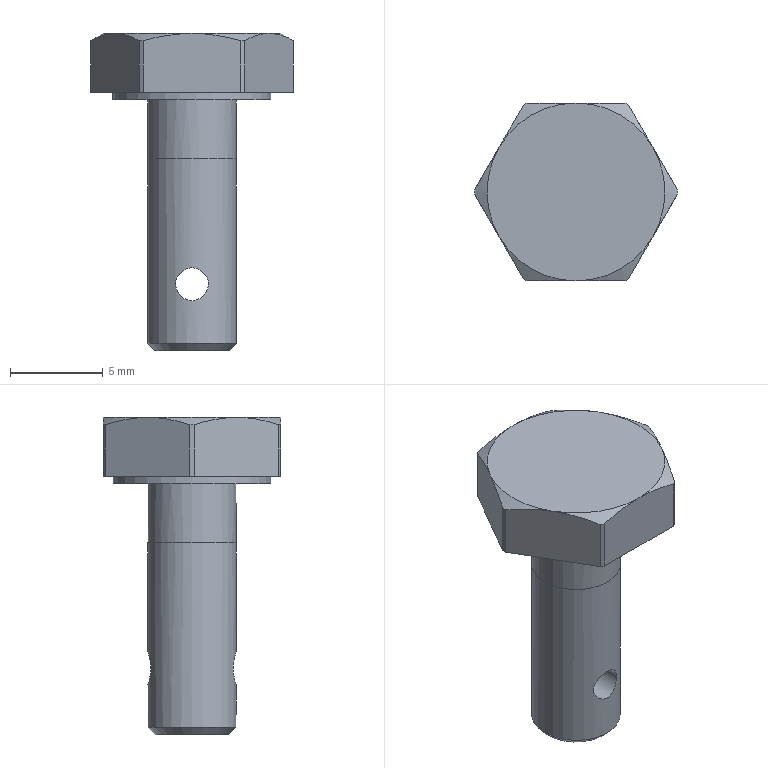Part | NX | features solid 2 | 1 solid | 27 faces | box 10.922 x 9.576 x 17.075 mm | volume 501.991 mm3 | cylinder 10 | plane 10 | cone 7 | commonest cylinder face diameters 10.922 x6 4.763 x2 1.778 x1 8.509 x1
STEP:
#1=CARTESIAN_POINT('',(0.,-2.381,-14.392));
#2=VERTEX_POINT('',#1);
#3=CARTESIAN_POINT('',(1.334,-2.037,-13.504));
#4=CARTESIAN_POINT('',(-0.00007358,-2.553,-14.836));
#5=CARTESIAN_POINT('',(-1.333,-2.037,-13.504));
#6=CARTESIAN_POINT('',(-0.0005145,-2.553,-12.169));
#7=CARTESIAN_POINT('',(1.334,-2.037,-13.504));
#8=CARTESIAN_POINT('',(-0.00007358,-2.553,-14.836));
#9=CARTESIAN_POINT('',(-1.333,-2.037,-13.504));
#10=B_SPLINE_CURVE_WITH_KNOTS('',3,(#3,#4,#5,#6,#7,#8,#9),.UNSPECIFIED.,.T.,.F.,(1,1,1,1,1,1,1,1,1,1,1),(-0.004207,-0.002805,-0.001402,0.,0.001402,0.002805,0.004207,0.00561,0.007012,0.008414,0.009817),.UNSPECIFIED.);
#11=EDGE_CURVE('',#2,#2,#10,.T.);
#12=ORIENTED_EDGE('',*,*,#11,.T.);
#13=EDGE_LOOP('',(#12));
#14=FACE_BOUND('',#13,.T.);
#15=CARTESIAN_POINT('',(-2.381,0.,-6.756));
#16=VERTEX_POINT('',#15);
#17=CARTESIAN_POINT('',(-1.866,1.866,-6.756));
#18=CARTESIAN_POINT('',(-2.639,0.,-6.756));
#19=CARTESIAN_POINT('',(-1.866,-1.866,-6.756));
#20=CARTESIAN_POINT('',(0.,-2.639,-6.756));
#21=CARTESIAN_POINT('',(1.866,-1.866,-6.756));
#22=CARTESIAN_POINT('',(2.639,0.,-6.756));
#23=CARTESIAN_POINT('',(1.866,1.866,-6.756));
#24=CARTESIAN_POINT('',(0.,2.639,-6.756));
#25=CARTESIAN_POINT('',(-1.866,1.866,-6.756));
#26=CARTESIAN_POINT('',(-2.639,0.,-6.756));
#27=CARTESIAN_POINT('',(-1.866,-1.866,-6.756));
#28=B_SPLINE_CURVE_WITH_KNOTS('',3,(#17,#18,#19,#20,#21,#22,#23,#24,#25,#26,#27),.UNSPECIFIED.,.T.,.F.,(1,1,1,1,1,1,1,1,1,1,1,1,1,1,1),(-0.375,-0.25,-0.125,0.,0.125,0.25,0.375,0.5,0.625,0.75,0.875,1.,1.125,1.25,1.375),.UNSPECIFIED.);
#29=EDGE_CURVE('',#16,#16,#28,.T.);
#30=ORIENTED_EDGE('',*,*,#29,.F.);
#31=EDGE_LOOP('',(#30));
#32=FACE_BOUND('',#31,.T.);
#33=CARTESIAN_POINT('',(-2.381,0.,-16.694));
#34=VERTEX_POINT('',#33);
#35=CARTESIAN_POINT('',(0.,0.,-16.694));
#36=DIRECTION('',(0.,0.,-1.));
#37=DIRECTION('',(-1.,0.,0.));
#38=AXIS2_PLACEMENT_3D('',#35,#36,#37);
#39=CIRCLE('',#38,2.381);
#40=EDGE_CURVE('',#34,#34,#39,.T.);
#41=ORIENTED_EDGE('',*,*,#40,.F.);
#42=EDGE_LOOP('',(#41));
#43=FACE_BOUND('',#42,.T.);
#44=CARTESIAN_POINT('',(0.,2.381,-14.392));
#45=VERTEX_POINT('',#44);
#46=CARTESIAN_POINT('',(-1.334,2.037,-13.504));
#47=CARTESIAN_POINT('',(0.00007358,2.553,-14.836));
#48=CARTESIAN_POINT('',(1.333,2.037,-13.504));
#49=CARTESIAN_POINT('',(0.0005145,2.553,-12.169));
#50=CARTESIAN_POINT('',(-1.334,2.037,-13.504));
#51=CARTESIAN_POINT('',(0.00007358,2.553,-14.836));
#52=CARTESIAN_POINT('',(1.333,2.037,-13.504));
#53=B_SPLINE_CURVE_WITH_KNOTS('',3,(#46,#47,#48,#49,#50,#51,#52),.UNSPECIFIED.,.T.,.F.,(1,1,1,1,1,1,1,1,1,1,1),(-0.004207,-0.002805,-0.001402,0.,0.001402,0.002805,0.004207,0.00561,0.007012,0.008414,0.009817),.UNSPECIFIED.);
#54=EDGE_CURVE('',#45,#45,#53,.T.);
#55=ORIENTED_EDGE('',*,*,#54,.T.);
#56=EDGE_LOOP('',(#55));
#57=FACE_BOUND('',#56,.T.);
#58=CARTESIAN_POINT('',(0.,0.,0.));
#59=DIRECTION('',(0.,0.,-1.));
#60=DIRECTION('',(-1.,0.,0.));
#61=AXIS2_PLACEMENT_3D('',#58,#59,#60);
#62=CYLINDRICAL_SURFACE('',#61,2.381);
#63=ADVANCED_FACE('',(#14,#32,#43,#57),#62,.T.);
#64=CARTESIAN_POINT('',(-2.381,0.,-3.581));
#65=VERTEX_POINT('',#64);
#66=CARTESIAN_POINT('',(0.,0.,-3.581));
#67=DIRECTION('',(0.,0.,-1.));
#68=DIRECTION('',(-1.,0.,0.));
#69=AXIS2_PLACEMENT_3D('',#66,#67,#68);
#70=CIRCLE('',#69,2.381);
#71=EDGE_CURVE('',#65,#65,#70,.T.);
#72=ORIENTED_EDGE('',*,*,#71,.T.);
#73=EDGE_LOOP('',(#72));
#74=FACE_BOUND('',#73,.T.);
#75=ORIENTED_EDGE('',*,*,#29,.T.);
#76=EDGE_LOOP('',(#75));
#77=FACE_BOUND('',#76,.T.);
#78=CARTESIAN_POINT('',(0.,0.,0.));
#79=DIRECTION('',(0.,0.,-1.));
#80=DIRECTION('',(-1.,0.,0.));
#81=AXIS2_PLACEMENT_3D('',#78,#79,#80);
#82=CYLINDRICAL_SURFACE('',#81,2.381);
#83=ADVANCED_FACE('',(#74,#77),#82,.T.);
#84=CARTESIAN_POINT('',(2.627,4.788,-3.175));
#85=VERTEX_POINT('',#84);
#86=CARTESIAN_POINT('',(2.833,4.669,-3.175));
#87=VERTEX_POINT('',#86);
#88=CARTESIAN_POINT('',(0.,0.,-3.175));
#89=DIRECTION('',(0.,0.,-1.));
#90=DIRECTION('',(-1.,0.,0.));
#91=AXIS2_PLACEMENT_3D('',#88,#89,#90);
#92=CIRCLE('',#91,5.461);
#93=EDGE_CURVE('',#85,#87,#92,.T.);
#94=ORIENTED_EDGE('',*,*,#93,.F.);
#95=CARTESIAN_POINT('',(2.627,4.788,-0.3886));
#96=VERTEX_POINT('',#95);
#97=CARTESIAN_POINT('',(2.627,4.788,0.));
#98=DIRECTION('',(0.,0.,-1.));
#99=VECTOR('',#98,1000.);
#100=LINE('',#97,#99);
#101=EDGE_CURVE('',#85,#96,#100,.F.);
#102=ORIENTED_EDGE('',*,*,#101,.T.);
#103=CARTESIAN_POINT('',(2.833,4.669,-0.3886));
#104=VERTEX_POINT('',#103);
#105=CARTESIAN_POINT('',(0.,0.,-0.3886));
#106=DIRECTION('',(0.,0.,-1.));
#107=DIRECTION('',(-1.,0.,0.));
#108=AXIS2_PLACEMENT_3D('',#105,#106,#107);
#109=CIRCLE('',#108,5.461);
#110=EDGE_CURVE('',#96,#104,#109,.T.);
#111=ORIENTED_EDGE('',*,*,#110,.T.);
#112=CARTESIAN_POINT('',(2.833,4.669,0.));
#113=DIRECTION('',(0.,0.,-1.));
#114=VECTOR('',#113,1000.);
#115=LINE('',#112,#114);
#116=EDGE_CURVE('',#104,#87,#115,.T.);
#117=ORIENTED_EDGE('',*,*,#116,.T.);
#118=EDGE_LOOP('',(#94,#102,#111,#117));
#119=FACE_BOUND('',#118,.T.);
#120=CARTESIAN_POINT('',(0.,0.,0.));
#121=DIRECTION('',(0.,0.,-1.));
#122=DIRECTION('',(-1.,0.,0.));
#123=AXIS2_PLACEMENT_3D('',#120,#121,#122);
#124=CYLINDRICAL_SURFACE('',#123,5.461);
#125=ADVANCED_FACE('',(#119),#124,.T.);
#126=CARTESIAN_POINT('',(-2.833,4.669,-0.3886));
#127=VERTEX_POINT('',#126);
#128=CARTESIAN_POINT('',(-2.627,4.788,-0.3886));
#129=VERTEX_POINT('',#128);
#130=CARTESIAN_POINT('',(0.,0.,-0.3886));
#131=DIRECTION('',(0.,0.,-1.));
#132=DIRECTION('',(-1.,0.,0.));
#133=AXIS2_PLACEMENT_3D('',#130,#131,#132);
#134=CIRCLE('',#133,5.461);
#135=EDGE_CURVE('',#127,#129,#134,.T.);
#136=ORIENTED_EDGE('',*,*,#135,.T.);
#137=CARTESIAN_POINT('',(-2.627,4.788,-3.175));
#138=VERTEX_POINT('',#137);
#139=CARTESIAN_POINT('',(-2.627,4.788,0.));
#140=DIRECTION('',(0.,0.,-1.));
#141=VECTOR('',#140,1000.);
#142=LINE('',#139,#141);
#143=EDGE_CURVE('',#129,#138,#142,.T.);
#144=ORIENTED_EDGE('',*,*,#143,.T.);
#145=CARTESIAN_POINT('',(-2.833,4.669,-3.175));
#146=VERTEX_POINT('',#145);
#147=CARTESIAN_POINT('',(0.,0.,-3.175));
#148=DIRECTION('',(0.,0.,-1.));
#149=DIRECTION('',(-1.,0.,0.));
#150=AXIS2_PLACEMENT_3D('',#147,#148,#149);
#151=CIRCLE('',#150,5.461);
#152=EDGE_CURVE('',#146,#138,#151,.T.);
#153=ORIENTED_EDGE('',*,*,#152,.F.);
#154=CARTESIAN_POINT('',(-2.833,4.669,0.));
#155=DIRECTION('',(0.,0.,-1.));
#156=VECTOR('',#155,1000.);
#157=LINE('',#154,#156);
#158=EDGE_CURVE('',#146,#127,#157,.F.);
#159=ORIENTED_EDGE('',*,*,#158,.T.);
#160=EDGE_LOOP('',(#136,#144,#153,#159));
#161=FACE_BOUND('',#160,.T.);
#162=CARTESIAN_POINT('',(0.,0.,0.));
#163=DIRECTION('',(0.,0.,-1.));
#164=DIRECTION('',(-1.,0.,0.));
#165=AXIS2_PLACEMENT_3D('',#162,#163,#164);
#166=CYLINDRICAL_SURFACE('',#165,5.461);
#167=ADVANCED_FACE('',(#161),#166,.T.);
#168=CARTESIAN_POINT('',(-5.46,-0.1193,-0.3886));
#169=VERTEX_POINT('',#168);
#170=CARTESIAN_POINT('',(-5.46,0.1193,-0.3886));
#171=VERTEX_POINT('',#170);
#172=CARTESIAN_POINT('',(0.,0.,-0.3886));
#173=DIRECTION('',(0.,0.,-1.));
#174=DIRECTION('',(-1.,0.,0.));
#175=AXIS2_PLACEMENT_3D('',#172,#173,#174);
#176=CIRCLE('',#175,5.461);
#177=EDGE_CURVE('',#169,#171,#176,.T.);
#178=ORIENTED_EDGE('',*,*,#177,.T.);
#179=CARTESIAN_POINT('',(-5.46,0.1193,-3.175));
#180=VERTEX_POINT('',#179);
#181=CARTESIAN_POINT('',(-5.46,0.1193,0.));
#182=DIRECTION('',(0.,0.,-1.));
#183=VECTOR('',#182,1000.);
#184=LINE('',#181,#183);
#185=EDGE_CURVE('',#171,#180,#184,.T.);
#186=ORIENTED_EDGE('',*,*,#185,.T.);
#187=CARTESIAN_POINT('',(-5.46,-0.1193,-3.175));
#188=VERTEX_POINT('',#187);
#189=CARTESIAN_POINT('',(0.,0.,-3.175));
#190=DIRECTION('',(0.,0.,-1.));
#191=DIRECTION('',(-1.,0.,0.));
#192=AXIS2_PLACEMENT_3D('',#189,#190,#191);
#193=CIRCLE('',#192,5.461);
#194=EDGE_CURVE('',#188,#180,#193,.T.);
#195=ORIENTED_EDGE('',*,*,#194,.F.);
#196=CARTESIAN_POINT('',(-5.46,-0.1193,0.));
#197=DIRECTION('',(0.,0.,-1.));
#198=VECTOR('',#197,1000.);
#199=LINE('',#196,#198);
#200=EDGE_CURVE('',#188,#169,#199,.F.);
#201=ORIENTED_EDGE('',*,*,#200,.T.);
#202=EDGE_LOOP('',(#178,#186,#195,#201));
#203=FACE_BOUND('',#202,.T.);
#204=CARTESIAN_POINT('',(0.,0.,0.));
#205=DIRECTION('',(0.,0.,-1.));
#206=DIRECTION('',(-1.,0.,0.));
#207=AXIS2_PLACEMENT_3D('',#204,#205,#206);
#208=CYLINDRICAL_SURFACE('',#207,5.461);
#209=ADVANCED_FACE('',(#203),#208,.T.);
#210=CARTESIAN_POINT('',(-2.627,-4.788,-0.3886));
#211=VERTEX_POINT('',#210);
#212=CARTESIAN_POINT('',(-2.833,-4.669,-0.3886));
#213=VERTEX_POINT('',#212);
#214=CARTESIAN_POINT('',(0.,0.,-0.3886));
#215=DIRECTION('',(0.,0.,-1.));
#216=DIRECTION('',(-1.,0.,0.));
#217=AXIS2_PLACEMENT_3D('',#214,#215,#216);
#218=CIRCLE('',#217,5.461);
#219=EDGE_CURVE('',#211,#213,#218,.T.);
#220=ORIENTED_EDGE('',*,*,#219,.T.);
#221=CARTESIAN_POINT('',(-2.833,-4.669,-3.175));
#222=VERTEX_POINT('',#221);
#223=CARTESIAN_POINT('',(-2.833,-4.669,0.));
#224=DIRECTION('',(0.,0.,-1.));
#225=VECTOR('',#224,1000.);
#226=LINE('',#223,#225);
#227=EDGE_CURVE('',#213,#222,#226,.T.);
#228=ORIENTED_EDGE('',*,*,#227,.T.);
#229=CARTESIAN_POINT('',(-2.627,-4.788,-3.175));
#230=VERTEX_POINT('',#229);
#231=CARTESIAN_POINT('',(0.,0.,-3.175));
#232=DIRECTION('',(0.,0.,-1.));
#233=DIRECTION('',(-1.,0.,0.));
#234=AXIS2_PLACEMENT_3D('',#231,#232,#233);
#235=CIRCLE('',#234,5.461);
#236=EDGE_CURVE('',#230,#222,#235,.T.);
#237=ORIENTED_EDGE('',*,*,#236,.F.);
#238=CARTESIAN_POINT('',(-2.627,-4.788,0.));
#239=DIRECTION('',(0.,0.,-1.));
#240=VECTOR('',#239,1000.);
#241=LINE('',#238,#240);
#242=EDGE_CURVE('',#230,#211,#241,.F.);
#243=ORIENTED_EDGE('',*,*,#242,.T.);
#244=EDGE_LOOP('',(#220,#228,#237,#243));
#245=FACE_BOUND('',#244,.T.);
#246=CARTESIAN_POINT('',(0.,0.,0.));
#247=DIRECTION('',(0.,0.,-1.));
#248=DIRECTION('',(-1.,0.,0.));
#249=AXIS2_PLACEMENT_3D('',#246,#247,#248);
#250=CYLINDRICAL_SURFACE('',#249,5.461);
#251=ADVANCED_FACE('',(#245),#250,.T.);
#252=CARTESIAN_POINT('',(2.833,-4.669,-0.3886));
#253=VERTEX_POINT('',#252);
#254=CARTESIAN_POINT('',(2.627,-4.788,-0.3886));
#255=VERTEX_POINT('',#254);
#256=CARTESIAN_POINT('',(0.,0.,-0.3886));
#257=DIRECTION('',(0.,0.,-1.));
#258=DIRECTION('',(-1.,0.,0.));
#259=AXIS2_PLACEMENT_3D('',#256,#257,#258);
#260=CIRCLE('',#259,5.461);
#261=EDGE_CURVE('',#253,#255,#260,.T.);
#262=ORIENTED_EDGE('',*,*,#261,.T.);
#263=CARTESIAN_POINT('',(2.627,-4.788,-3.175));
#264=VERTEX_POINT('',#263);
#265=CARTESIAN_POINT('',(2.627,-4.788,0.));
#266=DIRECTION('',(0.,0.,-1.));
#267=VECTOR('',#266,1000.);
#268=LINE('',#265,#267);
#269=EDGE_CURVE('',#255,#264,#268,.T.);
#270=ORIENTED_EDGE('',*,*,#269,.T.);
#271=CARTESIAN_POINT('',(2.833,-4.669,-3.175));
#272=VERTEX_POINT('',#271);
#273=CARTESIAN_POINT('',(0.,0.,-3.175));
#274=DIRECTION('',(0.,0.,-1.));
#275=DIRECTION('',(-1.,0.,0.));
#276=AXIS2_PLACEMENT_3D('',#273,#274,#275);
#277=CIRCLE('',#276,5.461);
#278=EDGE_CURVE('',#272,#264,#277,.T.);
#279=ORIENTED_EDGE('',*,*,#278,.F.);
#280=CARTESIAN_POINT('',(2.833,-4.669,0.));
#281=DIRECTION('',(0.,0.,-1.));
#282=VECTOR('',#281,1000.);
#283=LINE('',#280,#282);
#284=EDGE_CURVE('',#272,#253,#283,.F.);
#285=ORIENTED_EDGE('',*,*,#284,.T.);
#286=EDGE_LOOP('',(#262,#270,#279,#285));
#287=FACE_BOUND('',#286,.T.);
#288=CARTESIAN_POINT('',(0.,0.,0.));
#289=DIRECTION('',(0.,0.,-1.));
#290=DIRECTION('',(-1.,0.,0.));
#291=AXIS2_PLACEMENT_3D('',#288,#289,#290);
#292=CYLINDRICAL_SURFACE('',#291,5.461);
#293=ADVANCED_FACE('',(#287),#292,.T.);
#294=ORIENTED_EDGE('',*,*,#110,.F.);
#295=CARTESIAN_POINT('',(0.,4.788,0.));
#296=VERTEX_POINT('',#295);
#297=CARTESIAN_POINT('',(0.,4.788,0.));
#298=CARTESIAN_POINT('',(0.8868,4.788,0.));
#299=CARTESIAN_POINT('',(1.776,4.788,-0.1525));
#300=CARTESIAN_POINT('',(2.627,4.788,-0.3886));
#301=B_SPLINE_CURVE_WITH_KNOTS('',3,(#297,#298,#299,#300),.UNSPECIFIED.,.F.,.F.,(4,4),(0.007722,0.01038),.UNSPECIFIED.);
#302=EDGE_CURVE('',#96,#296,#301,.F.);
#303=ORIENTED_EDGE('',*,*,#302,.T.);
#304=CARTESIAN_POINT('',(4.146,2.394,0.));
#305=VERTEX_POINT('',#304);
#306=CARTESIAN_POINT('',(0.,0.,0.));
#307=DIRECTION('',(0.,0.,-1.));
#308=DIRECTION('',(-1.,0.,0.));
#309=AXIS2_PLACEMENT_3D('',#306,#307,#308);
#310=CIRCLE('',#309,4.788);
#311=EDGE_CURVE('',#296,#305,#310,.T.);
#312=ORIENTED_EDGE('',*,*,#311,.T.);
#313=CARTESIAN_POINT('',(4.146,2.394,0.));
#314=CARTESIAN_POINT('',(3.703,3.163,0.));
#315=CARTESIAN_POINT('',(3.262,3.925,-0.1503));
#316=CARTESIAN_POINT('',(2.833,4.669,-0.3886));
#317=B_SPLINE_CURVE_WITH_KNOTS('',3,(#313,#314,#315,#316),.UNSPECIFIED.,.F.,.F.,(4,4),(0.002655,0.005296),.UNSPECIFIED.);
#318=EDGE_CURVE('',#305,#104,#317,.T.);
#319=ORIENTED_EDGE('',*,*,#318,.T.);
#320=EDGE_LOOP('',(#294,#303,#312,#319));
#321=FACE_BOUND('',#320,.T.);
#322=CARTESIAN_POINT('',(0.,0.,-0.3886));
#323=DIRECTION('',(0.,0.,-1.));
#324=DIRECTION('',(-1.,0.,0.));
#325=AXIS2_PLACEMENT_3D('',#322,#323,#324);
#326=CONICAL_SURFACE('',#325,5.461,1.047);
#327=ADVANCED_FACE('',(#321),#326,.T.);
#328=CARTESIAN_POINT('',(-4.146,2.394,0.));
#329=VERTEX_POINT('',#328);
#330=CARTESIAN_POINT('',(0.,0.,0.));
#331=DIRECTION('',(0.,0.,-1.));
#332=DIRECTION('',(-1.,0.,0.));
#333=AXIS2_PLACEMENT_3D('',#330,#331,#332);
#334=CIRCLE('',#333,4.788);
#335=EDGE_CURVE('',#329,#296,#334,.T.);
#336=ORIENTED_EDGE('',*,*,#335,.T.);
#337=CARTESIAN_POINT('',(-2.627,4.788,-0.3886));
#338=CARTESIAN_POINT('',(-1.77,4.788,-0.1508));
#339=CARTESIAN_POINT('',(-0.8866,4.788,0.));
#340=CARTESIAN_POINT('',(0.,4.788,0.));
#341=B_SPLINE_CURVE_WITH_KNOTS('',3,(#337,#338,#339,#340),.UNSPECIFIED.,.F.,.F.,(4,4),(0.005068,0.007722),.UNSPECIFIED.);
#342=EDGE_CURVE('',#296,#129,#341,.F.);
#343=ORIENTED_EDGE('',*,*,#342,.T.);
#344=ORIENTED_EDGE('',*,*,#135,.F.);
#345=CARTESIAN_POINT('',(-2.833,4.669,-0.3886));
#346=CARTESIAN_POINT('',(-3.264,3.923,-0.1495));
#347=CARTESIAN_POINT('',(-3.7,3.167,0.));
#348=CARTESIAN_POINT('',(-4.146,2.394,0.));
#349=B_SPLINE_CURVE_WITH_KNOTS('',3,(#345,#346,#347,#348),.UNSPECIFIED.,.F.,.F.,(4,4),(0.00000074,0.002655),.UNSPECIFIED.);
#350=EDGE_CURVE('',#127,#329,#349,.T.);
#351=ORIENTED_EDGE('',*,*,#350,.T.);
#352=EDGE_LOOP('',(#336,#343,#344,#351));
#353=FACE_BOUND('',#352,.T.);
#354=CARTESIAN_POINT('',(0.,0.,-0.3886));
#355=DIRECTION('',(0.,0.,-1.));
#356=DIRECTION('',(-1.,0.,0.));
#357=AXIS2_PLACEMENT_3D('',#354,#355,#356);
#358=CONICAL_SURFACE('',#357,5.461,1.047);
#359=ADVANCED_FACE('',(#353),#358,.T.);
#360=CARTESIAN_POINT('',(-4.146,-2.394,0.));
#361=VERTEX_POINT('',#360);
#362=CARTESIAN_POINT('',(0.,0.,0.));
#363=DIRECTION('',(0.,0.,-1.));
#364=DIRECTION('',(-1.,0.,0.));
#365=AXIS2_PLACEMENT_3D('',#362,#363,#364);
#366=CIRCLE('',#365,4.788);
#367=EDGE_CURVE('',#361,#329,#366,.T.);
#368=ORIENTED_EDGE('',*,*,#367,.T.);
#369=CARTESIAN_POINT('',(-4.146,2.394,0.));
#370=CARTESIAN_POINT('',(-4.59,1.625,0.));
#371=CARTESIAN_POINT('',(-5.031,0.8625,-0.1503));
#372=CARTESIAN_POINT('',(-5.46,0.1193,-0.3886));
#373=B_SPLINE_CURVE_WITH_KNOTS('',3,(#369,#370,#371,#372),.UNSPECIFIED.,.F.,.F.,(4,4),(0.002655,0.005296),.UNSPECIFIED.);
#374=EDGE_CURVE('',#329,#171,#373,.T.);
#375=ORIENTED_EDGE('',*,*,#374,.T.);
#376=ORIENTED_EDGE('',*,*,#177,.F.);
#377=CARTESIAN_POINT('',(-5.46,-0.1193,-0.3886));
#378=CARTESIAN_POINT('',(-5.029,-0.8651,-0.1495));
#379=CARTESIAN_POINT('',(-4.593,-1.621,0.));
#380=CARTESIAN_POINT('',(-4.146,-2.394,0.));
#381=B_SPLINE_CURVE_WITH_KNOTS('',3,(#377,#378,#379,#380),.UNSPECIFIED.,.F.,.F.,(4,4),(0.00000074,0.002655),.UNSPECIFIED.);
#382=EDGE_CURVE('',#169,#361,#381,.T.);
#383=ORIENTED_EDGE('',*,*,#382,.T.);
#384=EDGE_LOOP('',(#368,#375,#376,#383));
#385=FACE_BOUND('',#384,.T.);
#386=CARTESIAN_POINT('',(0.,0.,-0.3886));
#387=DIRECTION('',(0.,0.,-1.));
#388=DIRECTION('',(-1.,0.,0.));
#389=AXIS2_PLACEMENT_3D('',#386,#387,#388);
#390=CONICAL_SURFACE('',#389,5.461,1.047);
#391=ADVANCED_FACE('',(#385),#390,.T.);
#392=CARTESIAN_POINT('',(0.,-4.788,0.));
#393=VERTEX_POINT('',#392);
#394=CARTESIAN_POINT('',(0.,0.,0.));
#395=DIRECTION('',(0.,0.,-1.));
#396=DIRECTION('',(-1.,0.,0.));
#397=AXIS2_PLACEMENT_3D('',#394,#395,#396);
#398=CIRCLE('',#397,4.788);
#399=EDGE_CURVE('',#393,#361,#398,.T.);
#400=ORIENTED_EDGE('',*,*,#399,.T.);
#401=CARTESIAN_POINT('',(-4.146,-2.394,0.));
#402=CARTESIAN_POINT('',(-3.703,-3.163,0.));
#403=CARTESIAN_POINT('',(-3.262,-3.925,-0.1503));
#404=CARTESIAN_POINT('',(-2.833,-4.669,-0.3886));
#405=B_SPLINE_CURVE_WITH_KNOTS('',3,(#401,#402,#403,#404),.UNSPECIFIED.,.F.,.F.,(4,4),(0.002655,0.005296),.UNSPECIFIED.);
#406=EDGE_CURVE('',#361,#213,#405,.T.);
#407=ORIENTED_EDGE('',*,*,#406,.T.);
#408=ORIENTED_EDGE('',*,*,#219,.F.);
#409=CARTESIAN_POINT('',(-2.627,-4.788,-0.3886));
#410=CARTESIAN_POINT('',(-1.77,-4.788,-0.1508));
#411=CARTESIAN_POINT('',(-0.8866,-4.788,0.));
#412=CARTESIAN_POINT('',(0.,-4.788,0.));
#413=B_SPLINE_CURVE_WITH_KNOTS('',3,(#409,#410,#411,#412),.UNSPECIFIED.,.F.,.F.,(4,4),(0.005068,0.007722),.UNSPECIFIED.);
#414=EDGE_CURVE('',#211,#393,#413,.T.);
#415=ORIENTED_EDGE('',*,*,#414,.T.);
#416=EDGE_LOOP('',(#400,#407,#408,#415));
#417=FACE_BOUND('',#416,.T.);
#418=CARTESIAN_POINT('',(0.,0.,-0.3886));
#419=DIRECTION('',(0.,0.,-1.));
#420=DIRECTION('',(-1.,0.,0.));
#421=AXIS2_PLACEMENT_3D('',#418,#419,#420);
#422=CONICAL_SURFACE('',#421,5.461,1.047);
#423=ADVANCED_FACE('',(#417),#422,.T.);
#424=CARTESIAN_POINT('',(4.146,-2.394,0.));
#425=VERTEX_POINT('',#424);
#426=CARTESIAN_POINT('',(0.,0.,0.));
#427=DIRECTION('',(0.,0.,-1.));
#428=DIRECTION('',(-1.,0.,0.));
#429=AXIS2_PLACEMENT_3D('',#426,#427,#428);
#430=CIRCLE('',#429,4.788);
#431=EDGE_CURVE('',#425,#393,#430,.T.);
#432=ORIENTED_EDGE('',*,*,#431,.T.);
#433=CARTESIAN_POINT('',(0.,-4.788,0.));
#434=CARTESIAN_POINT('',(0.8868,-4.788,0.));
#435=CARTESIAN_POINT('',(1.776,-4.788,-0.1525));
#436=CARTESIAN_POINT('',(2.627,-4.788,-0.3886));
#437=B_SPLINE_CURVE_WITH_KNOTS('',3,(#433,#434,#435,#436),.UNSPECIFIED.,.F.,.F.,(4,4),(0.007722,0.01038),.UNSPECIFIED.);
#438=EDGE_CURVE('',#393,#255,#437,.T.);
#439=ORIENTED_EDGE('',*,*,#438,.T.);
#440=ORIENTED_EDGE('',*,*,#261,.F.);
#441=CARTESIAN_POINT('',(2.833,-4.669,-0.3886));
#442=CARTESIAN_POINT('',(3.264,-3.923,-0.1495));
#443=CARTESIAN_POINT('',(3.7,-3.167,0.));
#444=CARTESIAN_POINT('',(4.146,-2.394,0.));
#445=B_SPLINE_CURVE_WITH_KNOTS('',3,(#441,#442,#443,#444),.UNSPECIFIED.,.F.,.F.,(4,4),(0.00000074,0.002655),.UNSPECIFIED.);
#446=EDGE_CURVE('',#253,#425,#445,.T.);
#447=ORIENTED_EDGE('',*,*,#446,.T.);
#448=EDGE_LOOP('',(#432,#439,#440,#447));
#449=FACE_BOUND('',#448,.T.);
#450=CARTESIAN_POINT('',(0.,0.,-0.3886));
#451=DIRECTION('',(0.,0.,-1.));
#452=DIRECTION('',(-1.,0.,0.));
#453=AXIS2_PLACEMENT_3D('',#450,#451,#452);
#454=CONICAL_SURFACE('',#453,5.461,1.047);
#455=ADVANCED_FACE('',(#449),#454,.T.);
#456=ORIENTED_EDGE('',*,*,#152,.T.);
#457=CARTESIAN_POINT('',(4.255,4.788,-3.175));
#458=DIRECTION('',(1.,0.,0.));
#459=VECTOR('',#458,1000.);
#460=LINE('',#457,#459);
#461=EDGE_CURVE('',#138,#85,#460,.T.);
#462=ORIENTED_EDGE('',*,*,#461,.T.);
#463=ORIENTED_EDGE('',*,*,#93,.T.);
#464=CARTESIAN_POINT('',(5.46,0.1193,-3.175));
#465=VERTEX_POINT('',#464);
#466=CARTESIAN_POINT('',(5.21,0.5517,-3.175));
#467=DIRECTION('',(0.5,-0.866,0.));
#468=VECTOR('',#467,1000.);
#469=LINE('',#466,#468);
#470=EDGE_CURVE('',#87,#465,#469,.T.);
#471=ORIENTED_EDGE('',*,*,#470,.T.);
#472=CARTESIAN_POINT('',(5.46,-0.1193,-3.175));
#473=VERTEX_POINT('',#472);
#474=CARTESIAN_POINT('',(0.,0.,-3.175));
#475=DIRECTION('',(0.,0.,-1.));
#476=DIRECTION('',(-1.,0.,0.));
#477=AXIS2_PLACEMENT_3D('',#474,#475,#476);
#478=CIRCLE('',#477,5.461);
#479=EDGE_CURVE('',#465,#473,#478,.T.);
#480=ORIENTED_EDGE('',*,*,#479,.T.);
#481=CARTESIAN_POINT('',(5.21,-0.5517,-3.175));
#482=DIRECTION('',(-0.5,-0.866,0.));
#483=VECTOR('',#482,1000.);
#484=LINE('',#481,#483);
#485=EDGE_CURVE('',#473,#272,#484,.T.);
#486=ORIENTED_EDGE('',*,*,#485,.T.);
#487=ORIENTED_EDGE('',*,*,#278,.T.);
#488=CARTESIAN_POINT('',(4.255,-4.788,-3.175));
#489=DIRECTION('',(-1.,0.,0.));
#490=VECTOR('',#489,1000.);
#491=LINE('',#488,#490);
#492=EDGE_CURVE('',#264,#230,#491,.T.);
#493=ORIENTED_EDGE('',*,*,#492,.T.);
#494=ORIENTED_EDGE('',*,*,#236,.T.);
#495=CARTESIAN_POINT('',(-3.083,-4.236,-3.175));
#496=DIRECTION('',(-0.5,0.866,0.));
#497=VECTOR('',#496,1000.);
#498=LINE('',#495,#497);
#499=EDGE_CURVE('',#222,#188,#498,.T.);
#500=ORIENTED_EDGE('',*,*,#499,.T.);
#501=ORIENTED_EDGE('',*,*,#194,.T.);
#502=CARTESIAN_POINT('',(-3.083,4.236,-3.175));
#503=DIRECTION('',(0.5,0.866,0.));
#504=VECTOR('',#503,1000.);
#505=LINE('',#502,#504);
#506=EDGE_CURVE('',#180,#146,#505,.T.);
#507=ORIENTED_EDGE('',*,*,#506,.T.);
#508=EDGE_LOOP('',(#456,#462,#463,#471,#480,#486,#487,#493,#494,#500,#501,#507));
#509=FACE_BOUND('',#508,.T.);
#510=CARTESIAN_POINT('',(-4.255,0.,-3.175));
#511=VERTEX_POINT('',#510);
#512=CARTESIAN_POINT('',(0.,0.,-3.175));
#513=DIRECTION('',(0.,0.,-1.));
#514=DIRECTION('',(-1.,0.,0.));
#515=AXIS2_PLACEMENT_3D('',#512,#513,#514);
#516=CIRCLE('',#515,4.255);
#517=EDGE_CURVE('',#511,#511,#516,.T.);
#518=ORIENTED_EDGE('',*,*,#517,.F.);
#519=EDGE_LOOP('',(#518));
#520=FACE_BOUND('',#519,.T.);
#521=CARTESIAN_POINT('',(4.255,0.,-3.175));
#522=DIRECTION('',(0.,0.,-1.));
#523=DIRECTION('',(-1.,0.,0.));
#524=AXIS2_PLACEMENT_3D('',#521,#522,#523);
#525=PLANE('',#524);
#526=ADVANCED_FACE('',(#509,#520),#525,.T.);
#527=CARTESIAN_POINT('',(5.46,0.1193,-0.3886));
#528=VERTEX_POINT('',#527);
#529=CARTESIAN_POINT('',(5.46,-0.1193,-0.3886));
#530=VERTEX_POINT('',#529);
#531=CARTESIAN_POINT('',(0.,0.,-0.3886));
#532=DIRECTION('',(0.,0.,-1.));
#533=DIRECTION('',(-1.,0.,0.));
#534=AXIS2_PLACEMENT_3D('',#531,#532,#533);
#535=CIRCLE('',#534,5.461);
#536=EDGE_CURVE('',#528,#530,#535,.T.);
#537=ORIENTED_EDGE('',*,*,#536,.T.);
#538=CARTESIAN_POINT('',(5.46,-0.1193,0.));
#539=DIRECTION('',(0.,0.,-1.));
#540=VECTOR('',#539,1000.);
#541=LINE('',#538,#540);
#542=EDGE_CURVE('',#530,#473,#541,.T.);
#543=ORIENTED_EDGE('',*,*,#542,.T.);
#544=ORIENTED_EDGE('',*,*,#479,.F.);
#545=CARTESIAN_POINT('',(5.46,0.1193,0.));
#546=DIRECTION('',(0.,0.,-1.));
#547=VECTOR('',#546,1000.);
#548=LINE('',#545,#547);
#549=EDGE_CURVE('',#465,#528,#548,.F.);
#550=ORIENTED_EDGE('',*,*,#549,.T.);
#551=EDGE_LOOP('',(#537,#543,#544,#550));
#552=FACE_BOUND('',#551,.T.);
#553=CARTESIAN_POINT('',(0.,0.,0.));
#554=DIRECTION('',(0.,0.,-1.));
#555=DIRECTION('',(-1.,0.,0.));
#556=AXIS2_PLACEMENT_3D('',#553,#554,#555);
#557=CYLINDRICAL_SURFACE('',#556,5.461);
#558=ADVANCED_FACE('',(#552),#557,.T.);
#559=CARTESIAN_POINT('',(0.,0.,0.));
#560=DIRECTION('',(0.,0.,-1.));
#561=DIRECTION('',(-1.,0.,0.));
#562=AXIS2_PLACEMENT_3D('',#559,#560,#561);
#563=CIRCLE('',#562,4.788);
#564=EDGE_CURVE('',#305,#425,#563,.T.);
#565=ORIENTED_EDGE('',*,*,#564,.T.);
#566=CARTESIAN_POINT('',(4.146,-2.394,0.));
#567=CARTESIAN_POINT('',(4.59,-1.625,0.));
#568=CARTESIAN_POINT('',(5.031,-0.8625,-0.1503));
#569=CARTESIAN_POINT('',(5.46,-0.1193,-0.3886));
#570=B_SPLINE_CURVE_WITH_KNOTS('',3,(#566,#567,#568,#569),.UNSPECIFIED.,.F.,.F.,(4,4),(0.002655,0.005296),.UNSPECIFIED.);
#571=EDGE_CURVE('',#425,#530,#570,.T.);
#572=ORIENTED_EDGE('',*,*,#571,.T.);
#573=ORIENTED_EDGE('',*,*,#536,.F.);
#574=CARTESIAN_POINT('',(5.46,0.1193,-0.3886));
#575=CARTESIAN_POINT('',(5.029,0.8651,-0.1495));
#576=CARTESIAN_POINT('',(4.593,1.621,0.));
#577=CARTESIAN_POINT('',(4.146,2.394,0.));
#578=B_SPLINE_CURVE_WITH_KNOTS('',3,(#574,#575,#576,#577),.UNSPECIFIED.,.F.,.F.,(4,4),(0.00000074,0.002655),.UNSPECIFIED.);
#579=EDGE_CURVE('',#528,#305,#578,.T.);
#580=ORIENTED_EDGE('',*,*,#579,.T.);
#581=EDGE_LOOP('',(#565,#572,#573,#580));
#582=FACE_BOUND('',#581,.T.);
#583=CARTESIAN_POINT('',(0.,0.,-0.3886));
#584=DIRECTION('',(0.,0.,-1.));
#585=DIRECTION('',(-1.,0.,0.));
#586=AXIS2_PLACEMENT_3D('',#583,#584,#585);
#587=CONICAL_SURFACE('',#586,5.461,1.047);
#588=ADVANCED_FACE('',(#582),#587,.T.);
#589=ORIENTED_EDGE('',*,*,#335,.F.);
#590=ORIENTED_EDGE('',*,*,#367,.F.);
#591=ORIENTED_EDGE('',*,*,#399,.F.);
#592=ORIENTED_EDGE('',*,*,#431,.F.);
#593=ORIENTED_EDGE('',*,*,#564,.F.);
#594=ORIENTED_EDGE('',*,*,#311,.F.);
#595=EDGE_LOOP('',(#589,#590,#591,#592,#593,#594));
#596=FACE_BOUND('',#595,.T.);
#597=CARTESIAN_POINT('',(4.788,0.,0.));
#598=DIRECTION('',(0.,0.,1.));
#599=DIRECTION('',(1.,0.,0.));
#600=AXIS2_PLACEMENT_3D('',#597,#598,#599);
#601=PLANE('',#600);
#602=ADVANCED_FACE('',(#596),#601,.T.);
#603=CARTESIAN_POINT('',(-2.,0.,-17.075));
#604=VERTEX_POINT('',#603);
#605=CARTESIAN_POINT('',(0.,0.,-17.075));
#606=DIRECTION('',(0.,0.,-1.));
#607=DIRECTION('',(-1.,0.,0.));
#608=AXIS2_PLACEMENT_3D('',#605,#606,#607);
#609=CIRCLE('',#608,2.);
#610=EDGE_CURVE('',#604,#604,#609,.T.);
#611=ORIENTED_EDGE('',*,*,#610,.T.);
#612=EDGE_LOOP('',(#611));
#613=FACE_BOUND('',#612,.T.);
#614=CARTESIAN_POINT('',(0.,0.,-17.075));
#615=DIRECTION('',(0.,0.,-1.));
#616=DIRECTION('',(-1.,0.,0.));
#617=AXIS2_PLACEMENT_3D('',#614,#615,#616);
#618=PLANE('',#617);
#619=ADVANCED_FACE('',(#613),#618,.T.);
#620=ORIENTED_EDGE('',*,*,#40,.T.);
#621=EDGE_LOOP('',(#620));
#622=FACE_BOUND('',#621,.T.);
#623=ORIENTED_EDGE('',*,*,#610,.F.);
#624=EDGE_LOOP('',(#623));
#625=FACE_BOUND('',#624,.T.);
#626=CARTESIAN_POINT('',(0.,0.,-17.075));
#627=DIRECTION('',(0.,0.,1.));
#628=DIRECTION('',(1.,0.,0.));
#629=AXIS2_PLACEMENT_3D('',#626,#627,#628);
#630=CONICAL_SURFACE('',#629,2.,0.7854);
#631=ADVANCED_FACE('',(#622,#625),#630,.T.);
#632=CARTESIAN_POINT('',(-4.255,0.,-3.581));
#633=VERTEX_POINT('',#632);
#634=CARTESIAN_POINT('',(0.,0.,-3.581));
#635=DIRECTION('',(0.,0.,-1.));
#636=DIRECTION('',(-1.,0.,0.));
#637=AXIS2_PLACEMENT_3D('',#634,#635,#636);
#638=CIRCLE('',#637,4.255);
#639=EDGE_CURVE('',#633,#633,#638,.T.);
#640=ORIENTED_EDGE('',*,*,#639,.T.);
#641=EDGE_LOOP('',(#640));
#642=FACE_BOUND('',#641,.T.);
#643=ORIENTED_EDGE('',*,*,#71,.F.);
#644=EDGE_LOOP('',(#643));
#645=FACE_BOUND('',#644,.T.);
#646=CARTESIAN_POINT('',(2.381,0.,-3.581));
#647=DIRECTION('',(0.,0.,-1.));
#648=DIRECTION('',(-1.,0.,0.));
#649=AXIS2_PLACEMENT_3D('',#646,#647,#648);
#650=PLANE('',#649);
#651=ADVANCED_FACE('',(#642,#645),#650,.T.);
#652=ORIENTED_EDGE('',*,*,#517,.T.);
#653=EDGE_LOOP('',(#652));
#654=FACE_BOUND('',#653,.T.);
#655=ORIENTED_EDGE('',*,*,#639,.F.);
#656=EDGE_LOOP('',(#655));
#657=FACE_BOUND('',#656,.T.);
#658=CARTESIAN_POINT('',(0.,0.,0.));
#659=DIRECTION('',(0.,0.,-1.));
#660=DIRECTION('',(-1.,0.,0.));
#661=AXIS2_PLACEMENT_3D('',#658,#659,#660);
#662=CYLINDRICAL_SURFACE('',#661,4.255);
#663=ADVANCED_FACE('',(#654,#657),#662,.T.);
#664=ORIENTED_EDGE('',*,*,#470,.F.);
#665=ORIENTED_EDGE('',*,*,#116,.F.);
#666=ORIENTED_EDGE('',*,*,#318,.F.);
#667=ORIENTED_EDGE('',*,*,#579,.F.);
#668=ORIENTED_EDGE('',*,*,#549,.F.);
#669=EDGE_LOOP('',(#664,#665,#666,#667,#668));
#670=FACE_BOUND('',#669,.T.);
#671=CARTESIAN_POINT('',(5.529,0.,-18.783));
#672=DIRECTION('',(0.866,0.5,0.));
#673=DIRECTION('',(-0.5,0.866,0.));
#674=AXIS2_PLACEMENT_3D('',#671,#672,#673);
#675=PLANE('',#674);
#676=ADVANCED_FACE('',(#670),#675,.T.);
#677=ORIENTED_EDGE('',*,*,#485,.F.);
#678=ORIENTED_EDGE('',*,*,#542,.F.);
#679=ORIENTED_EDGE('',*,*,#571,.F.);
#680=ORIENTED_EDGE('',*,*,#446,.F.);
#681=ORIENTED_EDGE('',*,*,#284,.F.);
#682=EDGE_LOOP('',(#677,#678,#679,#680,#681));
#683=FACE_BOUND('',#682,.T.);
#684=CARTESIAN_POINT('',(2.764,-4.788,-18.783));
#685=DIRECTION('',(0.866,-0.5,0.));
#686=DIRECTION('',(0.5,0.866,0.));
#687=AXIS2_PLACEMENT_3D('',#684,#685,#686);
#688=PLANE('',#687);
#689=ADVANCED_FACE('',(#683),#688,.T.);
#690=ORIENTED_EDGE('',*,*,#492,.F.);
#691=ORIENTED_EDGE('',*,*,#269,.F.);
#692=ORIENTED_EDGE('',*,*,#438,.F.);
#693=ORIENTED_EDGE('',*,*,#414,.F.);
#694=ORIENTED_EDGE('',*,*,#242,.F.);
#695=EDGE_LOOP('',(#690,#691,#692,#693,#694));
#696=FACE_BOUND('',#695,.T.);
#697=CARTESIAN_POINT('',(-2.764,-4.788,-18.783));
#698=DIRECTION('',(0.,-1.,0.));
#699=DIRECTION('',(0.,0.,-1.));
#700=AXIS2_PLACEMENT_3D('',#697,#698,#699);
#701=PLANE('',#700);
#702=ADVANCED_FACE('',(#696),#701,.T.);
#703=ORIENTED_EDGE('',*,*,#499,.F.);
#704=ORIENTED_EDGE('',*,*,#227,.F.);
#705=ORIENTED_EDGE('',*,*,#406,.F.);
#706=ORIENTED_EDGE('',*,*,#382,.F.);
#707=ORIENTED_EDGE('',*,*,#200,.F.);
#708=EDGE_LOOP('',(#703,#704,#705,#706,#707));
#709=FACE_BOUND('',#708,.T.);
#710=CARTESIAN_POINT('',(-5.529,0.,-18.783));
#711=DIRECTION('',(-0.866,-0.5,0.));
#712=DIRECTION('',(0.5,-0.866,0.));
#713=AXIS2_PLACEMENT_3D('',#710,#711,#712);
#714=PLANE('',#713);
#715=ADVANCED_FACE('',(#709),#714,.T.);
#716=ORIENTED_EDGE('',*,*,#506,.F.);
#717=ORIENTED_EDGE('',*,*,#185,.F.);
#718=ORIENTED_EDGE('',*,*,#374,.F.);
#719=ORIENTED_EDGE('',*,*,#350,.F.);
#720=ORIENTED_EDGE('',*,*,#158,.F.);
#721=EDGE_LOOP('',(#716,#717,#718,#719,#720));
#722=FACE_BOUND('',#721,.T.);
#723=CARTESIAN_POINT('',(-2.764,4.788,-18.783));
#724=DIRECTION('',(-0.866,0.5,0.));
#725=DIRECTION('',(-0.5,-0.866,0.));
#726=AXIS2_PLACEMENT_3D('',#723,#724,#725);
#727=PLANE('',#726);
#728=ADVANCED_FACE('',(#722),#727,.T.);
#729=ORIENTED_EDGE('',*,*,#461,.F.);
#730=ORIENTED_EDGE('',*,*,#143,.F.);
#731=ORIENTED_EDGE('',*,*,#342,.F.);
#732=ORIENTED_EDGE('',*,*,#302,.F.);
#733=ORIENTED_EDGE('',*,*,#101,.F.);
#734=EDGE_LOOP('',(#729,#730,#731,#732,#733));
#735=FACE_BOUND('',#734,.T.);
#736=CARTESIAN_POINT('',(2.764,4.788,-18.783));
#737=DIRECTION('',(0.,1.,0.));
#738=DIRECTION('',(0.,0.,1.));
#739=AXIS2_PLACEMENT_3D('',#736,#737,#738);
#740=PLANE('',#739);
#741=ADVANCED_FACE('',(#735),#740,.T.);
#742=ORIENTED_EDGE('',*,*,#54,.F.);
#743=EDGE_LOOP('',(#742));
#744=FACE_BOUND('',#743,.T.);
#745=ORIENTED_EDGE('',*,*,#11,.F.);
#746=EDGE_LOOP('',(#745));
#747=FACE_BOUND('',#746,.T.);
#748=CARTESIAN_POINT('',(0.,5.267,-13.503));
#749=DIRECTION('',(0.,-1.,0.));
#750=DIRECTION('',(0.,0.,-1.));
#751=AXIS2_PLACEMENT_3D('',#748,#749,#750);
#752=CYLINDRICAL_SURFACE('',#751,0.889);
#753=ADVANCED_FACE('',(#744,#747),#752,.F.);
#754=CLOSED_SHELL('',(#63,#83,#125,#167,#209,#251,#293,#327,#359,#391,#423,#455,#526,#558,#588,#602,#619,#631,#651,#663,#676,#689,#702,#715,#728,#741,#753));
#755=MANIFOLD_SOLID_BREP('',#754);
#756=(LENGTH_UNIT()NAMED_UNIT(*)SI_UNIT(.MILLI.,.METRE.));
#757=UNCERTAINTY_MEASURE_WITH_UNIT(LENGTH_MEASURE(0.0508),#756,'','');
#758=(NAMED_UNIT(*)PLANE_ANGLE_UNIT()SI_UNIT($,.RADIAN.));
#759=(NAMED_UNIT(*)SI_UNIT($,.STERADIAN.)SOLID_ANGLE_UNIT());
#760=(GEOMETRIC_REPRESENTATION_CONTEXT(3)GLOBAL_UNCERTAINTY_ASSIGNED_CONTEXT((#757))GLOBAL_UNIT_ASSIGNED_CONTEXT((#756,#758,#759))REPRESENTATION_CONTEXT('',''));
#761=ADVANCED_BREP_SHAPE_REPRESENTATION('',(#755),#760);